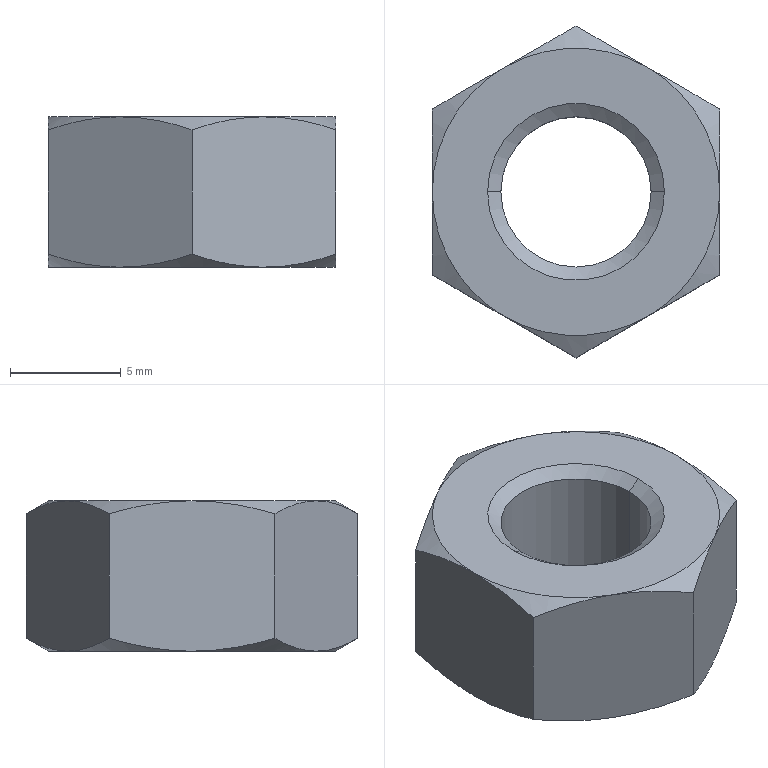Part | STEP file | Produce dryer cooling section-hex nut style 1_am_B18.2.4.1M - Hex nut, Style 1, M8 x 1.25 | 1 solid | 28 faces | box 13 x 15.011 x 6.8 mm | volume 737.453 mm3 | cone 16 | plane 8 | cylinder 4 | commonest cylinder face diameters 6.8 x2 8 x2
STEP:
#1=CARTESIAN_POINT('',(-4.,0.,-6.8));
#2=VERTEX_POINT('',#1);
#3=CARTESIAN_POINT('',(4.,0.,-6.8));
#4=VERTEX_POINT('',#3);
#5=CARTESIAN_POINT('',(0.,0.,-6.8));
#6=DIRECTION('',(0.,0.,1.));
#7=DIRECTION('',(-1.,0.,0.));
#8=AXIS2_PLACEMENT_3D('',#5,#6,#7);
#9=CIRCLE('',#8,4.);
#10=EDGE_CURVE('',#2,#4,#9,.T.);
#11=ORIENTED_EDGE('',*,*,#10,.F.);
#12=CARTESIAN_POINT('',(-4.,0.,-6.775));
#13=VERTEX_POINT('',#12);
#14=CARTESIAN_POINT('',(-4.,0.,-25.038));
#15=DIRECTION('',(0.,0.,1.));
#16=VECTOR('',#15,1000.);
#17=LINE('',#14,#16);
#18=EDGE_CURVE('',#2,#13,#17,.T.);
#19=ORIENTED_EDGE('',*,*,#18,.T.);
#20=CARTESIAN_POINT('',(4.,0.,-6.775));
#21=VERTEX_POINT('',#20);
#22=CARTESIAN_POINT('',(0.,0.,-6.775));
#23=DIRECTION('',(0.,0.,1.));
#24=DIRECTION('',(1.,0.,0.));
#25=AXIS2_PLACEMENT_3D('',#22,#23,#24);
#26=CIRCLE('',#25,4.);
#27=EDGE_CURVE('',#13,#21,#26,.T.);
#28=ORIENTED_EDGE('',*,*,#27,.T.);
#29=CARTESIAN_POINT('',(4.,0.,-25.038));
#30=DIRECTION('',(0.,0.,1.));
#31=VECTOR('',#30,1000.);
#32=LINE('',#29,#31);
#33=EDGE_CURVE('',#4,#21,#32,.T.);
#34=ORIENTED_EDGE('',*,*,#33,.F.);
#35=EDGE_LOOP('',(#11,#19,#28,#34));
#36=FACE_OUTER_BOUND('',#35,.T.);
#37=CARTESIAN_POINT('',(0.,0.,-25.038));
#38=DIRECTION('',(0.,0.,1.));
#39=DIRECTION('',(1.,0.,0.));
#40=AXIS2_PLACEMENT_3D('',#37,#38,#39);
#41=CYLINDRICAL_SURFACE('',#40,4.);
#42=ADVANCED_FACE('',(#36),#41,.F.);
#43=CARTESIAN_POINT('',(-3.4,0.,-6.354));
#44=VERTEX_POINT('',#43);
#45=CARTESIAN_POINT('',(3.4,0.,-6.354));
#46=VERTEX_POINT('',#45);
#47=CARTESIAN_POINT('',(0.,0.,-6.354));
#48=DIRECTION('',(0.,0.,1.));
#49=DIRECTION('',(-1.,0.,0.));
#50=AXIS2_PLACEMENT_3D('',#47,#48,#49);
#51=CIRCLE('',#50,3.4);
#52=EDGE_CURVE('',#44,#46,#51,.T.);
#53=ORIENTED_EDGE('',*,*,#52,.T.);
#54=CARTESIAN_POINT('',(4.,0.,-6.775));
#55=DIRECTION('',(0.8192,0.,-0.5736));
#56=VECTOR('',#55,1000.);
#57=LINE('',#54,#56);
#58=EDGE_CURVE('',#46,#21,#57,.T.);
#59=ORIENTED_EDGE('',*,*,#58,.T.);
#60=ORIENTED_EDGE('',*,*,#27,.F.);
#61=CARTESIAN_POINT('',(-4.,0.,-6.775));
#62=DIRECTION('',(-0.8192,0.,-0.5736));
#63=VECTOR('',#62,1000.);
#64=LINE('',#61,#63);
#65=EDGE_CURVE('',#44,#13,#64,.T.);
#66=ORIENTED_EDGE('',*,*,#65,.F.);
#67=EDGE_LOOP('',(#53,#59,#60,#66));
#68=FACE_OUTER_BOUND('',#67,.T.);
#69=CARTESIAN_POINT('',(0.,0.,-6.775));
#70=DIRECTION('',(0.,0.,-1.));
#71=DIRECTION('',(-1.,0.,0.));
#72=AXIS2_PLACEMENT_3D('',#69,#70,#71);
#73=CONICAL_SURFACE('',#72,4.,0.9599);
#74=ADVANCED_FACE('',(#68),#73,.F.);
#75=CARTESIAN_POINT('',(3.4,0.,-0.4201));
#76=VERTEX_POINT('',#75);
#77=CARTESIAN_POINT('',(-3.4,0.,-0.4201));
#78=VERTEX_POINT('',#77);
#79=CARTESIAN_POINT('',(0.,0.,-0.4201));
#80=DIRECTION('',(0.,0.,-1.));
#81=DIRECTION('',(1.,0.,0.));
#82=AXIS2_PLACEMENT_3D('',#79,#80,#81);
#83=CIRCLE('',#82,3.4);
#84=EDGE_CURVE('',#76,#78,#83,.T.);
#85=ORIENTED_EDGE('',*,*,#84,.T.);
#86=CARTESIAN_POINT('',(-4.,0.,0.));
#87=VERTEX_POINT('',#86);
#88=CARTESIAN_POINT('',(-3.34,0.,-0.4621));
#89=DIRECTION('',(-0.8192,0.,0.5736));
#90=VECTOR('',#89,1000.);
#91=LINE('',#88,#90);
#92=EDGE_CURVE('',#78,#87,#91,.T.);
#93=ORIENTED_EDGE('',*,*,#92,.T.);
#94=CARTESIAN_POINT('',(4.,0.,0.));
#95=VERTEX_POINT('',#94);
#96=CARTESIAN_POINT('',(0.,0.,0.));
#97=DIRECTION('',(0.,0.,1.));
#98=DIRECTION('',(1.,0.,0.));
#99=AXIS2_PLACEMENT_3D('',#96,#97,#98);
#100=CIRCLE('',#99,4.);
#101=EDGE_CURVE('',#87,#95,#100,.T.);
#102=ORIENTED_EDGE('',*,*,#101,.T.);
#103=CARTESIAN_POINT('',(3.34,0.,-0.4621));
#104=DIRECTION('',(0.8192,0.,0.5736));
#105=VECTOR('',#104,1000.);
#106=LINE('',#103,#105);
#107=EDGE_CURVE('',#76,#95,#106,.T.);
#108=ORIENTED_EDGE('',*,*,#107,.F.);
#109=EDGE_LOOP('',(#85,#93,#102,#108));
#110=FACE_OUTER_BOUND('',#109,.T.);
#111=CARTESIAN_POINT('',(0.,0.,-0.4621));
#112=DIRECTION('',(0.,0.,1.));
#113=DIRECTION('',(1.,0.,0.));
#114=AXIS2_PLACEMENT_3D('',#111,#112,#113);
#115=CONICAL_SURFACE('',#114,3.34,0.9599);
#116=ADVANCED_FACE('',(#110),#115,.F.);
#117=ORIENTED_EDGE('',*,*,#52,.F.);
#118=CARTESIAN_POINT('',(-3.4,0.,-6.8));
#119=DIRECTION('',(0.,0.,1.));
#120=VECTOR('',#119,1000.);
#121=LINE('',#118,#120);
#122=EDGE_CURVE('',#44,#78,#121,.T.);
#123=ORIENTED_EDGE('',*,*,#122,.T.);
#124=ORIENTED_EDGE('',*,*,#84,.F.);
#125=CARTESIAN_POINT('',(3.4,0.,-6.8));
#126=DIRECTION('',(0.,0.,1.));
#127=VECTOR('',#126,1000.);
#128=LINE('',#125,#127);
#129=EDGE_CURVE('',#46,#76,#128,.T.);
#130=ORIENTED_EDGE('',*,*,#129,.F.);
#131=EDGE_LOOP('',(#117,#123,#124,#130));
#132=FACE_OUTER_BOUND('',#131,.T.);
#133=CARTESIAN_POINT('',(0.,0.,-6.8));
#134=DIRECTION('',(0.,0.,1.));
#135=DIRECTION('',(1.,0.,0.));
#136=AXIS2_PLACEMENT_3D('',#133,#134,#135);
#137=CYLINDRICAL_SURFACE('',#136,3.4);
#138=ADVANCED_FACE('',(#132),#137,.F.);
#139=ORIENTED_EDGE('',*,*,#122,.F.);
#140=CARTESIAN_POINT('',(0.,0.,-6.354));
#141=DIRECTION('',(0.,0.,1.));
#142=DIRECTION('',(-1.,0.,0.));
#143=AXIS2_PLACEMENT_3D('',#140,#141,#142);
#144=CIRCLE('',#143,3.4);
#145=EDGE_CURVE('',#46,#44,#144,.T.);
#146=ORIENTED_EDGE('',*,*,#145,.F.);
#147=ORIENTED_EDGE('',*,*,#129,.T.);
#148=CARTESIAN_POINT('',(0.,0.,-0.4201));
#149=DIRECTION('',(0.,0.,-1.));
#150=DIRECTION('',(1.,0.,0.));
#151=AXIS2_PLACEMENT_3D('',#148,#149,#150);
#152=CIRCLE('',#151,3.4);
#153=EDGE_CURVE('',#78,#76,#152,.T.);
#154=ORIENTED_EDGE('',*,*,#153,.F.);
#155=EDGE_LOOP('',(#139,#146,#147,#154));
#156=FACE_OUTER_BOUND('',#155,.T.);
#157=CARTESIAN_POINT('',(0.,0.,-6.8));
#158=DIRECTION('',(0.,0.,1.));
#159=DIRECTION('',(1.,0.,0.));
#160=AXIS2_PLACEMENT_3D('',#157,#158,#159);
#161=CYLINDRICAL_SURFACE('',#160,3.4);
#162=ADVANCED_FACE('',(#156),#161,.F.);
#163=CARTESIAN_POINT('',(-6.5,3.753,-6.219));
#164=VERTEX_POINT('',#163);
#165=CARTESIAN_POINT('',(-6.5,3.753,-0.5806));
#166=VERTEX_POINT('',#165);
#167=CARTESIAN_POINT('',(-6.5,3.753,-6.8));
#168=DIRECTION('',(0.,0.,1.));
#169=VECTOR('',#168,1000.);
#170=LINE('',#167,#169);
#171=EDGE_CURVE('',#164,#166,#170,.T.);
#172=ORIENTED_EDGE('',*,*,#171,.T.);
#173=CARTESIAN_POINT('',(-3.25,5.629,0.));
#174=VERTEX_POINT('',#173);
#175=CARTESIAN_POINT('',(-6.5,3.753,-0.5806));
#176=CARTESIAN_POINT('',(-5.968,4.06,-0.4033));
#177=CARTESIAN_POINT('',(-5.433,4.369,-0.2573));
#178=CARTESIAN_POINT('',(-4.351,4.994,-0.05533));
#179=CARTESIAN_POINT('',(-3.804,5.309,0.));
#180=CARTESIAN_POINT('',(-3.25,5.629,0.));
#181=B_SPLINE_CURVE_WITH_KNOTS('',3,(#175,#176,#177,#178,#179,#180),.UNSPECIFIED.,.F.,.F.,(4,2,4),(0.000000238,0.001899,0.003797),.UNSPECIFIED.);
#182=EDGE_CURVE('',#166,#174,#181,.T.);
#183=ORIENTED_EDGE('',*,*,#182,.T.);
#184=CARTESIAN_POINT('',(0.,7.506,-0.5806));
#185=VERTEX_POINT('',#184);
#186=CARTESIAN_POINT('',(-3.25,5.629,0.));
#187=CARTESIAN_POINT('',(-2.974,5.788,0.));
#188=CARTESIAN_POINT('',(-2.697,5.948,-0.01372));
#189=CARTESIAN_POINT('',(-2.149,6.265,-0.06683));
#190=CARTESIAN_POINT('',(-1.877,6.422,-0.1062));
#191=CARTESIAN_POINT('',(-1.065,6.891,-0.2578));
#192=CARTESIAN_POINT('',(-0.5303,7.199,-0.4038));
#193=CARTESIAN_POINT('',(0.,7.506,-0.5806));
#194=B_SPLINE_CURVE_WITH_KNOTS('',3,(#186,#187,#188,#189,#190,#191,#192,#193),.UNSPECIFIED.,.F.,.F.,(4,2,2,4),(0.003797,0.004743,0.005689,0.00758),.UNSPECIFIED.);
#195=EDGE_CURVE('',#174,#185,#194,.T.);
#196=ORIENTED_EDGE('',*,*,#195,.T.);
#197=CARTESIAN_POINT('',(0.,7.506,-6.219));
#198=VERTEX_POINT('',#197);
#199=CARTESIAN_POINT('',(0.,7.506,-6.8));
#200=DIRECTION('',(0.,0.,1.));
#201=VECTOR('',#200,1000.);
#202=LINE('',#199,#201);
#203=EDGE_CURVE('',#198,#185,#202,.T.);
#204=ORIENTED_EDGE('',*,*,#203,.F.);
#205=CARTESIAN_POINT('',(-3.25,5.629,-6.8));
#206=VERTEX_POINT('',#205);
#207=CARTESIAN_POINT('',(-3.25,5.629,-6.8));
#208=CARTESIAN_POINT('',(-2.974,5.788,-6.8));
#209=CARTESIAN_POINT('',(-2.697,5.948,-6.786));
#210=CARTESIAN_POINT('',(-2.149,6.265,-6.733));
#211=CARTESIAN_POINT('',(-1.877,6.422,-6.694));
#212=CARTESIAN_POINT('',(-1.065,6.891,-6.542));
#213=CARTESIAN_POINT('',(-0.5303,7.199,-6.396));
#214=CARTESIAN_POINT('',(0.,7.506,-6.219));
#215=B_SPLINE_CURVE_WITH_KNOTS('',3,(#207,#208,#209,#210,#211,#212,#213,#214),.UNSPECIFIED.,.F.,.F.,(4,2,2,4),(0.003797,0.004743,0.005689,0.00758),.UNSPECIFIED.);
#216=EDGE_CURVE('',#206,#198,#215,.T.);
#217=ORIENTED_EDGE('',*,*,#216,.F.);
#218=CARTESIAN_POINT('',(-6.5,3.753,-6.219));
#219=CARTESIAN_POINT('',(-5.968,4.06,-6.397));
#220=CARTESIAN_POINT('',(-5.433,4.369,-6.543));
#221=CARTESIAN_POINT('',(-4.351,4.994,-6.745));
#222=CARTESIAN_POINT('',(-3.804,5.309,-6.8));
#223=CARTESIAN_POINT('',(-3.25,5.629,-6.8));
#224=B_SPLINE_CURVE_WITH_KNOTS('',3,(#218,#219,#220,#221,#222,#223),.UNSPECIFIED.,.F.,.F.,(4,2,4),(0.000000238,0.001899,0.003797),.UNSPECIFIED.);
#225=EDGE_CURVE('',#164,#206,#224,.T.);
#226=ORIENTED_EDGE('',*,*,#225,.F.);
#227=EDGE_LOOP('',(#172,#183,#196,#204,#217,#226));
#228=FACE_OUTER_BOUND('',#227,.T.);
#229=CARTESIAN_POINT('',(0.,7.506,-6.8));
#230=DIRECTION('',(-0.5,0.866,0.));
#231=DIRECTION('',(-0.866,-0.5,0.));
#232=AXIS2_PLACEMENT_3D('',#229,#230,#231);
#233=PLANE('',#232);
#234=ADVANCED_FACE('',(#228),#233,.T.);
#235=ORIENTED_EDGE('',*,*,#203,.T.);
#236=CARTESIAN_POINT('',(3.25,5.629,0.));
#237=VERTEX_POINT('',#236);
#238=CARTESIAN_POINT('',(0.,7.506,-0.5806));
#239=CARTESIAN_POINT('',(0.5317,7.199,-0.4033));
#240=CARTESIAN_POINT('',(1.067,6.889,-0.2573));
#241=CARTESIAN_POINT('',(2.149,6.265,-0.05533));
#242=CARTESIAN_POINT('',(2.696,5.949,0.));
#243=CARTESIAN_POINT('',(3.25,5.629,0.));
#244=B_SPLINE_CURVE_WITH_KNOTS('',3,(#238,#239,#240,#241,#242,#243),.UNSPECIFIED.,.F.,.F.,(4,2,4),(0.000000238,0.001899,0.003797),.UNSPECIFIED.);
#245=EDGE_CURVE('',#185,#237,#244,.T.);
#246=ORIENTED_EDGE('',*,*,#245,.T.);
#247=CARTESIAN_POINT('',(6.5,3.753,-0.5806));
#248=VERTEX_POINT('',#247);
#249=CARTESIAN_POINT('',(3.25,5.629,0.));
#250=CARTESIAN_POINT('',(3.526,5.47,0.));
#251=CARTESIAN_POINT('',(3.803,5.31,-0.01372));
#252=CARTESIAN_POINT('',(4.351,4.994,-0.06683));
#253=CARTESIAN_POINT('',(4.623,4.836,-0.1062));
#254=CARTESIAN_POINT('',(5.435,4.368,-0.2578));
#255=CARTESIAN_POINT('',(5.97,4.059,-0.4038));
#256=CARTESIAN_POINT('',(6.5,3.753,-0.5806));
#257=B_SPLINE_CURVE_WITH_KNOTS('',3,(#249,#250,#251,#252,#253,#254,#255,#256),.UNSPECIFIED.,.F.,.F.,(4,2,2,4),(0.003797,0.004743,0.005689,0.00758),.UNSPECIFIED.);
#258=EDGE_CURVE('',#237,#248,#257,.T.);
#259=ORIENTED_EDGE('',*,*,#258,.T.);
#260=CARTESIAN_POINT('',(6.5,3.753,-6.219));
#261=VERTEX_POINT('',#260);
#262=CARTESIAN_POINT('',(6.5,3.753,-6.8));
#263=DIRECTION('',(0.,0.,1.));
#264=VECTOR('',#263,1000.);
#265=LINE('',#262,#264);
#266=EDGE_CURVE('',#261,#248,#265,.T.);
#267=ORIENTED_EDGE('',*,*,#266,.F.);
#268=CARTESIAN_POINT('',(3.25,5.629,-6.8));
#269=VERTEX_POINT('',#268);
#270=CARTESIAN_POINT('',(3.25,5.629,-6.8));
#271=CARTESIAN_POINT('',(3.526,5.47,-6.8));
#272=CARTESIAN_POINT('',(3.803,5.31,-6.786));
#273=CARTESIAN_POINT('',(4.351,4.994,-6.733));
#274=CARTESIAN_POINT('',(4.623,4.836,-6.694));
#275=CARTESIAN_POINT('',(5.435,4.368,-6.542));
#276=CARTESIAN_POINT('',(5.97,4.059,-6.396));
#277=CARTESIAN_POINT('',(6.5,3.753,-6.219));
#278=B_SPLINE_CURVE_WITH_KNOTS('',3,(#270,#271,#272,#273,#274,#275,#276,#277),.UNSPECIFIED.,.F.,.F.,(4,2,2,4),(0.003797,0.004743,0.005689,0.00758),.UNSPECIFIED.);
#279=EDGE_CURVE('',#269,#261,#278,.T.);
#280=ORIENTED_EDGE('',*,*,#279,.F.);
#281=CARTESIAN_POINT('',(0.,7.506,-6.219));
#282=CARTESIAN_POINT('',(0.5317,7.199,-6.397));
#283=CARTESIAN_POINT('',(1.067,6.889,-6.543));
#284=CARTESIAN_POINT('',(2.149,6.265,-6.745));
#285=CARTESIAN_POINT('',(2.696,5.949,-6.8));
#286=CARTESIAN_POINT('',(3.25,5.629,-6.8));
#287=B_SPLINE_CURVE_WITH_KNOTS('',3,(#281,#282,#283,#284,#285,#286),.UNSPECIFIED.,.F.,.F.,(4,2,4),(0.000000238,0.001899,0.003797),.UNSPECIFIED.);
#288=EDGE_CURVE('',#198,#269,#287,.T.);
#289=ORIENTED_EDGE('',*,*,#288,.F.);
#290=EDGE_LOOP('',(#235,#246,#259,#267,#280,#289));
#291=FACE_OUTER_BOUND('',#290,.T.);
#292=CARTESIAN_POINT('',(6.5,3.753,-6.8));
#293=DIRECTION('',(0.5,0.866,0.));
#294=DIRECTION('',(-0.866,0.5,0.));
#295=AXIS2_PLACEMENT_3D('',#292,#293,#294);
#296=PLANE('',#295);
#297=ADVANCED_FACE('',(#291),#296,.T.);
#298=CARTESIAN_POINT('',(6.5,-3.753,-0.5806));
#299=VERTEX_POINT('',#298);
#300=CARTESIAN_POINT('',(6.5,0.,0.));
#301=VERTEX_POINT('',#300);
#302=CARTESIAN_POINT('',(6.5,-3.753,-0.5806));
#303=CARTESIAN_POINT('',(6.5,-3.142,-0.4044));
#304=CARTESIAN_POINT('',(6.5,-2.517,-0.2566));
#305=CARTESIAN_POINT('',(6.5,-1.264,-0.05451));
#306=CARTESIAN_POINT('',(6.5,-0.6342,0.));
#307=CARTESIAN_POINT('',(6.5,0.,0.));
#308=B_SPLINE_CURVE_WITH_KNOTS('',3,(#302,#303,#304,#305,#306,#307),.UNSPECIFIED.,.F.,.F.,(4,2,4),(0.006695,0.008594,0.01049),.UNSPECIFIED.);
#309=EDGE_CURVE('',#299,#301,#308,.T.);
#310=ORIENTED_EDGE('',*,*,#309,.F.);
#311=CARTESIAN_POINT('',(6.5,-3.753,-6.219));
#312=VERTEX_POINT('',#311);
#313=CARTESIAN_POINT('',(6.5,-3.753,-6.8));
#314=DIRECTION('',(0.,0.,1.));
#315=VECTOR('',#314,1000.);
#316=LINE('',#313,#315);
#317=EDGE_CURVE('',#312,#299,#316,.T.);
#318=ORIENTED_EDGE('',*,*,#317,.F.);
#319=CARTESIAN_POINT('',(6.5,0.,-6.8));
#320=VERTEX_POINT('',#319);
#321=CARTESIAN_POINT('',(6.5,-3.753,-6.219));
#322=CARTESIAN_POINT('',(6.5,-3.142,-6.396));
#323=CARTESIAN_POINT('',(6.5,-2.517,-6.543));
#324=CARTESIAN_POINT('',(6.5,-1.264,-6.745));
#325=CARTESIAN_POINT('',(6.5,-0.6342,-6.8));
#326=CARTESIAN_POINT('',(6.5,0.,-6.8));
#327=B_SPLINE_CURVE_WITH_KNOTS('',3,(#321,#322,#323,#324,#325,#326),.UNSPECIFIED.,.F.,.F.,(4,2,4),(0.006695,0.008594,0.01049),.UNSPECIFIED.);
#328=EDGE_CURVE('',#312,#320,#327,.T.);
#329=ORIENTED_EDGE('',*,*,#328,.T.);
#330=CARTESIAN_POINT('',(6.5,0.,-6.8));
#331=CARTESIAN_POINT('',(6.5,0.6345,-6.8));
#332=CARTESIAN_POINT('',(6.5,1.278,-6.744));
#333=CARTESIAN_POINT('',(6.5,2.531,-6.54));
#334=CARTESIAN_POINT('',(6.5,3.146,-6.395));
#335=CARTESIAN_POINT('',(6.5,3.753,-6.219));
#336=B_SPLINE_CURVE_WITH_KNOTS('',3,(#330,#331,#332,#333,#334,#335),.UNSPECIFIED.,.F.,.F.,(4,2,4),(0.01049,0.01239,0.01429),.UNSPECIFIED.);
#337=EDGE_CURVE('',#320,#261,#336,.T.);
#338=ORIENTED_EDGE('',*,*,#337,.T.);
#339=ORIENTED_EDGE('',*,*,#266,.T.);
#340=CARTESIAN_POINT('',(6.5,0.,0.));
#341=CARTESIAN_POINT('',(6.5,0.6345,0.));
#342=CARTESIAN_POINT('',(6.5,1.278,-0.05602));
#343=CARTESIAN_POINT('',(6.5,2.531,-0.2595));
#344=CARTESIAN_POINT('',(6.5,3.146,-0.4054));
#345=CARTESIAN_POINT('',(6.5,3.753,-0.5806));
#346=B_SPLINE_CURVE_WITH_KNOTS('',3,(#340,#341,#342,#343,#344,#345),.UNSPECIFIED.,.F.,.F.,(4,2,4),(0.01049,0.01239,0.01429),.UNSPECIFIED.);
#347=EDGE_CURVE('',#301,#248,#346,.T.);
#348=ORIENTED_EDGE('',*,*,#347,.F.);
#349=EDGE_LOOP('',(#310,#318,#329,#338,#339,#348));
#350=FACE_OUTER_BOUND('',#349,.T.);
#351=CARTESIAN_POINT('',(6.5,3.753,-6.8));
#352=DIRECTION('',(-1.,0.,0.));
#353=DIRECTION('',(0.,0.,1.));
#354=AXIS2_PLACEMENT_3D('',#351,#352,#353);
#355=PLANE('',#354);
#356=ADVANCED_FACE('',(#350),#355,.F.);
#357=ORIENTED_EDGE('',*,*,#317,.T.);
#358=CARTESIAN_POINT('',(3.25,-5.629,0.));
#359=VERTEX_POINT('',#358);
#360=CARTESIAN_POINT('',(6.5,-3.753,-0.5806));
#361=CARTESIAN_POINT('',(5.968,-4.06,-0.4033));
#362=CARTESIAN_POINT('',(5.433,-4.369,-0.2573));
#363=CARTESIAN_POINT('',(4.351,-4.994,-0.05533));
#364=CARTESIAN_POINT('',(3.804,-5.309,0.));
#365=CARTESIAN_POINT('',(3.25,-5.629,0.));
#366=B_SPLINE_CURVE_WITH_KNOTS('',3,(#360,#361,#362,#363,#364,#365),.UNSPECIFIED.,.F.,.F.,(4,2,4),(0.000000238,0.001899,0.003797),.UNSPECIFIED.);
#367=EDGE_CURVE('',#299,#359,#366,.T.);
#368=ORIENTED_EDGE('',*,*,#367,.T.);
#369=CARTESIAN_POINT('',(0.,-7.506,-0.5806));
#370=VERTEX_POINT('',#369);
#371=CARTESIAN_POINT('',(3.25,-5.629,0.));
#372=CARTESIAN_POINT('',(2.974,-5.788,0.));
#373=CARTESIAN_POINT('',(2.697,-5.948,-0.01372));
#374=CARTESIAN_POINT('',(2.149,-6.265,-0.06683));
#375=CARTESIAN_POINT('',(1.877,-6.422,-0.1062));
#376=CARTESIAN_POINT('',(1.065,-6.891,-0.2578));
#377=CARTESIAN_POINT('',(0.5303,-7.199,-0.4038));
#378=CARTESIAN_POINT('',(0.,-7.506,-0.5806));
#379=B_SPLINE_CURVE_WITH_KNOTS('',3,(#371,#372,#373,#374,#375,#376,#377,#378),.UNSPECIFIED.,.F.,.F.,(4,2,2,4),(0.003797,0.004743,0.005689,0.00758),.UNSPECIFIED.);
#380=EDGE_CURVE('',#359,#370,#379,.T.);
#381=ORIENTED_EDGE('',*,*,#380,.T.);
#382=CARTESIAN_POINT('',(0.,-7.506,-6.219));
#383=VERTEX_POINT('',#382);
#384=CARTESIAN_POINT('',(0.,-7.506,-6.8));
#385=DIRECTION('',(0.,0.,1.));
#386=VECTOR('',#385,1000.);
#387=LINE('',#384,#386);
#388=EDGE_CURVE('',#383,#370,#387,.T.);
#389=ORIENTED_EDGE('',*,*,#388,.F.);
#390=CARTESIAN_POINT('',(3.25,-5.629,-6.8));
#391=VERTEX_POINT('',#390);
#392=CARTESIAN_POINT('',(3.25,-5.629,-6.8));
#393=CARTESIAN_POINT('',(2.974,-5.788,-6.8));
#394=CARTESIAN_POINT('',(2.697,-5.948,-6.786));
#395=CARTESIAN_POINT('',(2.149,-6.265,-6.733));
#396=CARTESIAN_POINT('',(1.877,-6.422,-6.694));
#397=CARTESIAN_POINT('',(1.065,-6.891,-6.542));
#398=CARTESIAN_POINT('',(0.5303,-7.199,-6.396));
#399=CARTESIAN_POINT('',(0.,-7.506,-6.219));
#400=B_SPLINE_CURVE_WITH_KNOTS('',3,(#392,#393,#394,#395,#396,#397,#398,#399),.UNSPECIFIED.,.F.,.F.,(4,2,2,4),(0.003797,0.004743,0.005689,0.00758),.UNSPECIFIED.);
#401=EDGE_CURVE('',#391,#383,#400,.T.);
#402=ORIENTED_EDGE('',*,*,#401,.F.);
#403=CARTESIAN_POINT('',(6.5,-3.753,-6.219));
#404=CARTESIAN_POINT('',(5.968,-4.06,-6.397));
#405=CARTESIAN_POINT('',(5.433,-4.369,-6.543));
#406=CARTESIAN_POINT('',(4.351,-4.994,-6.745));
#407=CARTESIAN_POINT('',(3.804,-5.309,-6.8));
#408=CARTESIAN_POINT('',(3.25,-5.629,-6.8));
#409=B_SPLINE_CURVE_WITH_KNOTS('',3,(#403,#404,#405,#406,#407,#408),.UNSPECIFIED.,.F.,.F.,(4,2,4),(0.000000238,0.001899,0.003797),.UNSPECIFIED.);
#410=EDGE_CURVE('',#312,#391,#409,.T.);
#411=ORIENTED_EDGE('',*,*,#410,.F.);
#412=EDGE_LOOP('',(#357,#368,#381,#389,#402,#411));
#413=FACE_OUTER_BOUND('',#412,.T.);
#414=CARTESIAN_POINT('',(0.,-7.506,-6.8));
#415=DIRECTION('',(0.5,-0.866,0.));
#416=DIRECTION('',(0.866,0.5,0.));
#417=AXIS2_PLACEMENT_3D('',#414,#415,#416);
#418=PLANE('',#417);
#419=ADVANCED_FACE('',(#413),#418,.T.);
#420=ORIENTED_EDGE('',*,*,#388,.T.);
#421=CARTESIAN_POINT('',(-3.25,-5.629,0.));
#422=VERTEX_POINT('',#421);
#423=CARTESIAN_POINT('',(0.,-7.506,-0.5806));
#424=CARTESIAN_POINT('',(-0.5317,-7.199,-0.4033));
#425=CARTESIAN_POINT('',(-1.067,-6.889,-0.2573));
#426=CARTESIAN_POINT('',(-2.149,-6.265,-0.05533));
#427=CARTESIAN_POINT('',(-2.696,-5.949,0.));
#428=CARTESIAN_POINT('',(-3.25,-5.629,0.));
#429=B_SPLINE_CURVE_WITH_KNOTS('',3,(#423,#424,#425,#426,#427,#428),.UNSPECIFIED.,.F.,.F.,(4,2,4),(0.000000238,0.001899,0.003797),.UNSPECIFIED.);
#430=EDGE_CURVE('',#370,#422,#429,.T.);
#431=ORIENTED_EDGE('',*,*,#430,.T.);
#432=CARTESIAN_POINT('',(-6.5,-3.753,-0.5806));
#433=VERTEX_POINT('',#432);
#434=CARTESIAN_POINT('',(-3.25,-5.629,0.));
#435=CARTESIAN_POINT('',(-3.526,-5.47,0.));
#436=CARTESIAN_POINT('',(-3.803,-5.31,-0.01372));
#437=CARTESIAN_POINT('',(-4.351,-4.994,-0.06683));
#438=CARTESIAN_POINT('',(-4.623,-4.836,-0.1062));
#439=CARTESIAN_POINT('',(-5.435,-4.368,-0.2578));
#440=CARTESIAN_POINT('',(-5.97,-4.059,-0.4038));
#441=CARTESIAN_POINT('',(-6.5,-3.753,-0.5806));
#442=B_SPLINE_CURVE_WITH_KNOTS('',3,(#434,#435,#436,#437,#438,#439,#440,#441),.UNSPECIFIED.,.F.,.F.,(4,2,2,4),(0.003797,0.004743,0.005689,0.00758),.UNSPECIFIED.);
#443=EDGE_CURVE('',#422,#433,#442,.T.);
#444=ORIENTED_EDGE('',*,*,#443,.T.);
#445=CARTESIAN_POINT('',(-6.5,-3.753,-6.219));
#446=VERTEX_POINT('',#445);
#447=CARTESIAN_POINT('',(-6.5,-3.753,-6.8));
#448=DIRECTION('',(0.,0.,1.));
#449=VECTOR('',#448,1000.);
#450=LINE('',#447,#449);
#451=EDGE_CURVE('',#446,#433,#450,.T.);
#452=ORIENTED_EDGE('',*,*,#451,.F.);
#453=CARTESIAN_POINT('',(-3.25,-5.629,-6.8));
#454=VERTEX_POINT('',#453);
#455=CARTESIAN_POINT('',(-3.25,-5.629,-6.8));
#456=CARTESIAN_POINT('',(-3.526,-5.47,-6.8));
#457=CARTESIAN_POINT('',(-3.803,-5.31,-6.786));
#458=CARTESIAN_POINT('',(-4.351,-4.994,-6.733));
#459=CARTESIAN_POINT('',(-4.623,-4.836,-6.694));
#460=CARTESIAN_POINT('',(-5.435,-4.368,-6.542));
#461=CARTESIAN_POINT('',(-5.97,-4.059,-6.396));
#462=CARTESIAN_POINT('',(-6.5,-3.753,-6.219));
#463=B_SPLINE_CURVE_WITH_KNOTS('',3,(#455,#456,#457,#458,#459,#460,#461,#462),.UNSPECIFIED.,.F.,.F.,(4,2,2,4),(0.003797,0.004743,0.005689,0.00758),.UNSPECIFIED.);
#464=EDGE_CURVE('',#454,#446,#463,.T.);
#465=ORIENTED_EDGE('',*,*,#464,.F.);
#466=CARTESIAN_POINT('',(0.,-7.506,-6.219));
#467=CARTESIAN_POINT('',(-0.5317,-7.199,-6.397));
#468=CARTESIAN_POINT('',(-1.067,-6.889,-6.543));
#469=CARTESIAN_POINT('',(-2.149,-6.265,-6.745));
#470=CARTESIAN_POINT('',(-2.696,-5.949,-6.8));
#471=CARTESIAN_POINT('',(-3.25,-5.629,-6.8));
#472=B_SPLINE_CURVE_WITH_KNOTS('',3,(#466,#467,#468,#469,#470,#471),.UNSPECIFIED.,.F.,.F.,(4,2,4),(0.000000238,0.001899,0.003797),.UNSPECIFIED.);
#473=EDGE_CURVE('',#383,#454,#472,.T.);
#474=ORIENTED_EDGE('',*,*,#473,.F.);
#475=EDGE_LOOP('',(#420,#431,#444,#452,#465,#474));
#476=FACE_OUTER_BOUND('',#475,.T.);
#477=CARTESIAN_POINT('',(-6.5,-3.753,-6.8));
#478=DIRECTION('',(-0.5,-0.866,0.));
#479=DIRECTION('',(0.866,-0.5,0.));
#480=AXIS2_PLACEMENT_3D('',#477,#478,#479);
#481=PLANE('',#480);
#482=ADVANCED_FACE('',(#476),#481,.T.);
#483=ORIENTED_EDGE('',*,*,#451,.T.);
#484=CARTESIAN_POINT('',(-6.5,0.,0.));
#485=VERTEX_POINT('',#484);
#486=CARTESIAN_POINT('',(-6.5,-3.753,-0.5806));
#487=CARTESIAN_POINT('',(-6.5,-3.142,-0.4044));
#488=CARTESIAN_POINT('',(-6.5,-2.517,-0.2566));
#489=CARTESIAN_POINT('',(-6.5,-1.264,-0.05451));
#490=CARTESIAN_POINT('',(-6.5,-0.6342,0.));
#491=CARTESIAN_POINT('',(-6.5,0.,0.));
#492=B_SPLINE_CURVE_WITH_KNOTS('',3,(#486,#487,#488,#489,#490,#491),.UNSPECIFIED.,.F.,.F.,(4,2,4),(0.006695,0.008594,0.01049),.UNSPECIFIED.);
#493=EDGE_CURVE('',#433,#485,#492,.T.);
#494=ORIENTED_EDGE('',*,*,#493,.T.);
#495=CARTESIAN_POINT('',(-6.5,0.,0.));
#496=CARTESIAN_POINT('',(-6.5,0.6345,0.));
#497=CARTESIAN_POINT('',(-6.5,1.278,-0.05602));
#498=CARTESIAN_POINT('',(-6.5,2.531,-0.2595));
#499=CARTESIAN_POINT('',(-6.5,3.146,-0.4054));
#500=CARTESIAN_POINT('',(-6.5,3.753,-0.5806));
#501=B_SPLINE_CURVE_WITH_KNOTS('',3,(#495,#496,#497,#498,#499,#500),.UNSPECIFIED.,.F.,.F.,(4,2,4),(0.01049,0.01239,0.01429),.UNSPECIFIED.);
#502=EDGE_CURVE('',#485,#166,#501,.T.);
#503=ORIENTED_EDGE('',*,*,#502,.T.);
#504=ORIENTED_EDGE('',*,*,#171,.F.);
#505=CARTESIAN_POINT('',(-6.5,0.,-6.8));
#506=VERTEX_POINT('',#505);
#507=CARTESIAN_POINT('',(-6.5,0.,-6.8));
#508=CARTESIAN_POINT('',(-6.5,0.6345,-6.8));
#509=CARTESIAN_POINT('',(-6.5,1.278,-6.744));
#510=CARTESIAN_POINT('',(-6.5,2.531,-6.54));
#511=CARTESIAN_POINT('',(-6.5,3.146,-6.395));
#512=CARTESIAN_POINT('',(-6.5,3.753,-6.219));
#513=B_SPLINE_CURVE_WITH_KNOTS('',3,(#507,#508,#509,#510,#511,#512),.UNSPECIFIED.,.F.,.F.,(4,2,4),(0.01049,0.01239,0.01429),.UNSPECIFIED.);
#514=EDGE_CURVE('',#506,#164,#513,.T.);
#515=ORIENTED_EDGE('',*,*,#514,.F.);
#516=CARTESIAN_POINT('',(-6.5,-3.753,-6.219));
#517=CARTESIAN_POINT('',(-6.5,-3.142,-6.396));
#518=CARTESIAN_POINT('',(-6.5,-2.517,-6.543));
#519=CARTESIAN_POINT('',(-6.5,-1.264,-6.745));
#520=CARTESIAN_POINT('',(-6.5,-0.6342,-6.8));
#521=CARTESIAN_POINT('',(-6.5,0.,-6.8));
#522=B_SPLINE_CURVE_WITH_KNOTS('',3,(#516,#517,#518,#519,#520,#521),.UNSPECIFIED.,.F.,.F.,(4,2,4),(0.006695,0.008594,0.01049),.UNSPECIFIED.);
#523=EDGE_CURVE('',#446,#506,#522,.T.);
#524=ORIENTED_EDGE('',*,*,#523,.F.);
#525=EDGE_LOOP('',(#483,#494,#503,#504,#515,#524));
#526=FACE_OUTER_BOUND('',#525,.T.);
#527=CARTESIAN_POINT('',(-6.5,3.753,-6.8));
#528=DIRECTION('',(-1.,0.,0.));
#529=DIRECTION('',(0.,0.,1.));
#530=AXIS2_PLACEMENT_3D('',#527,#528,#529);
#531=PLANE('',#530);
#532=ADVANCED_FACE('',(#526),#531,.T.);
#533=CARTESIAN_POINT('',(0.,0.,0.));
#534=DIRECTION('',(0.,0.,1.));
#535=DIRECTION('',(1.,0.,0.));
#536=AXIS2_PLACEMENT_3D('',#533,#534,#535);
#537=CIRCLE('',#536,4.);
#538=EDGE_CURVE('',#95,#87,#537,.T.);
#539=ORIENTED_EDGE('',*,*,#538,.F.);
#540=ORIENTED_EDGE('',*,*,#101,.F.);
#541=EDGE_LOOP('',(#539,#540));
#542=FACE_BOUND('',#541,.T.);
#543=CARTESIAN_POINT('',(0.,0.,0.));
#544=DIRECTION('',(0.,0.,-1.));
#545=DIRECTION('',(-1.,0.,0.));
#546=AXIS2_PLACEMENT_3D('',#543,#544,#545);
#547=CIRCLE('',#546,6.5);
#548=EDGE_CURVE('',#485,#174,#547,.T.);
#549=ORIENTED_EDGE('',*,*,#548,.F.);
#550=CARTESIAN_POINT('',(0.,0.,0.));
#551=DIRECTION('',(0.,0.,-1.));
#552=DIRECTION('',(-1.,0.,0.));
#553=AXIS2_PLACEMENT_3D('',#550,#551,#552);
#554=CIRCLE('',#553,6.5);
#555=EDGE_CURVE('',#422,#485,#554,.T.);
#556=ORIENTED_EDGE('',*,*,#555,.F.);
#557=CARTESIAN_POINT('',(0.,0.,0.));
#558=DIRECTION('',(0.,0.,-1.));
#559=DIRECTION('',(-1.,0.,0.));
#560=AXIS2_PLACEMENT_3D('',#557,#558,#559);
#561=CIRCLE('',#560,6.5);
#562=EDGE_CURVE('',#359,#422,#561,.T.);
#563=ORIENTED_EDGE('',*,*,#562,.F.);
#564=CARTESIAN_POINT('',(0.,0.,0.));
#565=DIRECTION('',(0.,0.,-1.));
#566=DIRECTION('',(-1.,0.,0.));
#567=AXIS2_PLACEMENT_3D('',#564,#565,#566);
#568=CIRCLE('',#567,6.5);
#569=EDGE_CURVE('',#301,#359,#568,.T.);
#570=ORIENTED_EDGE('',*,*,#569,.F.);
#571=CARTESIAN_POINT('',(0.,0.,0.));
#572=DIRECTION('',(0.,0.,1.));
#573=DIRECTION('',(1.,0.,0.));
#574=AXIS2_PLACEMENT_3D('',#571,#572,#573);
#575=CIRCLE('',#574,6.5);
#576=EDGE_CURVE('',#301,#237,#575,.T.);
#577=ORIENTED_EDGE('',*,*,#576,.T.);
#578=CARTESIAN_POINT('',(0.,0.,0.));
#579=DIRECTION('',(0.,0.,-1.));
#580=DIRECTION('',(-1.,0.,0.));
#581=AXIS2_PLACEMENT_3D('',#578,#579,#580);
#582=CIRCLE('',#581,6.5);
#583=EDGE_CURVE('',#174,#237,#582,.T.);
#584=ORIENTED_EDGE('',*,*,#583,.F.);
#585=EDGE_LOOP('',(#549,#556,#563,#570,#577,#584));
#586=FACE_OUTER_BOUND('',#585,.T.);
#587=CARTESIAN_POINT('',(0.,7.506,0.));
#588=DIRECTION('',(0.,0.,-1.));
#589=DIRECTION('',(-1.,0.,0.));
#590=AXIS2_PLACEMENT_3D('',#587,#588,#589);
#591=PLANE('',#590);
#592=ADVANCED_FACE('',(#542,#586),#591,.F.);
#593=CARTESIAN_POINT('',(0.,0.,-6.8));
#594=DIRECTION('',(0.,0.,1.));
#595=DIRECTION('',(-1.,0.,0.));
#596=AXIS2_PLACEMENT_3D('',#593,#594,#595);
#597=CIRCLE('',#596,4.);
#598=EDGE_CURVE('',#4,#2,#597,.T.);
#599=ORIENTED_EDGE('',*,*,#598,.T.);
#600=ORIENTED_EDGE('',*,*,#10,.T.);
#601=EDGE_LOOP('',(#599,#600));
#602=FACE_BOUND('',#601,.T.);
#603=CARTESIAN_POINT('',(0.,0.,-6.8));
#604=DIRECTION('',(0.,0.,1.));
#605=DIRECTION('',(-1.,0.,0.));
#606=AXIS2_PLACEMENT_3D('',#603,#604,#605);
#607=CIRCLE('',#606,6.5);
#608=EDGE_CURVE('',#506,#454,#607,.T.);
#609=ORIENTED_EDGE('',*,*,#608,.F.);
#610=CARTESIAN_POINT('',(0.,0.,-6.8));
#611=DIRECTION('',(0.,0.,1.));
#612=DIRECTION('',(-1.,0.,0.));
#613=AXIS2_PLACEMENT_3D('',#610,#611,#612);
#614=CIRCLE('',#613,6.5);
#615=EDGE_CURVE('',#206,#506,#614,.T.);
#616=ORIENTED_EDGE('',*,*,#615,.F.);
#617=CARTESIAN_POINT('',(0.,0.,-6.8));
#618=DIRECTION('',(0.,0.,1.));
#619=DIRECTION('',(-1.,0.,0.));
#620=AXIS2_PLACEMENT_3D('',#617,#618,#619);
#621=CIRCLE('',#620,6.5);
#622=EDGE_CURVE('',#269,#206,#621,.T.);
#623=ORIENTED_EDGE('',*,*,#622,.F.);
#624=CARTESIAN_POINT('',(0.,0.,-6.8));
#625=DIRECTION('',(0.,0.,1.));
#626=DIRECTION('',(1.,0.,0.));
#627=AXIS2_PLACEMENT_3D('',#624,#625,#626);
#628=CIRCLE('',#627,6.5);
#629=EDGE_CURVE('',#320,#269,#628,.T.);
#630=ORIENTED_EDGE('',*,*,#629,.F.);
#631=CARTESIAN_POINT('',(0.,0.,-6.8));
#632=DIRECTION('',(0.,0.,1.));
#633=DIRECTION('',(-1.,0.,0.));
#634=AXIS2_PLACEMENT_3D('',#631,#632,#633);
#635=CIRCLE('',#634,6.5);
#636=EDGE_CURVE('',#391,#320,#635,.T.);
#637=ORIENTED_EDGE('',*,*,#636,.F.);
#638=CARTESIAN_POINT('',(0.,0.,-6.8));
#639=DIRECTION('',(0.,0.,1.));
#640=DIRECTION('',(-1.,0.,0.));
#641=AXIS2_PLACEMENT_3D('',#638,#639,#640);
#642=CIRCLE('',#641,6.5);
#643=EDGE_CURVE('',#454,#391,#642,.T.);
#644=ORIENTED_EDGE('',*,*,#643,.F.);
#645=EDGE_LOOP('',(#609,#616,#623,#630,#637,#644));
#646=FACE_OUTER_BOUND('',#645,.T.);
#647=CARTESIAN_POINT('',(0.,7.506,-6.8));
#648=DIRECTION('',(0.,0.,-1.));
#649=DIRECTION('',(-1.,0.,0.));
#650=AXIS2_PLACEMENT_3D('',#647,#648,#649);
#651=PLANE('',#650);
#652=ADVANCED_FACE('',(#602,#646),#651,.T.);
#653=ORIENTED_EDGE('',*,*,#225,.T.);
#654=ORIENTED_EDGE('',*,*,#615,.T.);
#655=ORIENTED_EDGE('',*,*,#514,.T.);
#656=EDGE_LOOP('',(#653,#654,#655));
#657=FACE_OUTER_BOUND('',#656,.T.);
#658=CARTESIAN_POINT('',(0.,0.,-6.8));
#659=DIRECTION('',(0.,0.,1.));
#660=DIRECTION('',(1.,0.,0.));
#661=AXIS2_PLACEMENT_3D('',#658,#659,#660);
#662=CONICAL_SURFACE('',#661,6.5,1.047);
#663=ADVANCED_FACE('',(#657),#662,.T.);
#664=ORIENTED_EDGE('',*,*,#216,.T.);
#665=ORIENTED_EDGE('',*,*,#288,.T.);
#666=ORIENTED_EDGE('',*,*,#622,.T.);
#667=EDGE_LOOP('',(#664,#665,#666));
#668=FACE_OUTER_BOUND('',#667,.T.);
#669=CARTESIAN_POINT('',(0.,0.,-6.8));
#670=DIRECTION('',(0.,0.,1.));
#671=DIRECTION('',(1.,0.,0.));
#672=AXIS2_PLACEMENT_3D('',#669,#670,#671);
#673=CONICAL_SURFACE('',#672,6.5,1.047);
#674=ADVANCED_FACE('',(#668),#673,.T.);
#675=ORIENTED_EDGE('',*,*,#279,.T.);
#676=ORIENTED_EDGE('',*,*,#337,.F.);
#677=ORIENTED_EDGE('',*,*,#629,.T.);
#678=EDGE_LOOP('',(#675,#676,#677));
#679=FACE_OUTER_BOUND('',#678,.T.);
#680=CARTESIAN_POINT('',(0.,0.,-6.8));
#681=DIRECTION('',(0.,0.,1.));
#682=DIRECTION('',(1.,0.,0.));
#683=AXIS2_PLACEMENT_3D('',#680,#681,#682);
#684=CONICAL_SURFACE('',#683,6.5,1.047);
#685=ADVANCED_FACE('',(#679),#684,.T.);
#686=ORIENTED_EDGE('',*,*,#410,.T.);
#687=ORIENTED_EDGE('',*,*,#636,.T.);
#688=ORIENTED_EDGE('',*,*,#328,.F.);
#689=EDGE_LOOP('',(#686,#687,#688));
#690=FACE_OUTER_BOUND('',#689,.T.);
#691=CARTESIAN_POINT('',(0.,0.,-6.8));
#692=DIRECTION('',(0.,0.,1.));
#693=DIRECTION('',(1.,0.,0.));
#694=AXIS2_PLACEMENT_3D('',#691,#692,#693);
#695=CONICAL_SURFACE('',#694,6.5,1.047);
#696=ADVANCED_FACE('',(#690),#695,.T.);
#697=ORIENTED_EDGE('',*,*,#401,.T.);
#698=ORIENTED_EDGE('',*,*,#473,.T.);
#699=ORIENTED_EDGE('',*,*,#643,.T.);
#700=EDGE_LOOP('',(#697,#698,#699));
#701=FACE_OUTER_BOUND('',#700,.T.);
#702=CARTESIAN_POINT('',(0.,0.,-6.8));
#703=DIRECTION('',(0.,0.,1.));
#704=DIRECTION('',(1.,0.,0.));
#705=AXIS2_PLACEMENT_3D('',#702,#703,#704);
#706=CONICAL_SURFACE('',#705,6.5,1.047);
#707=ADVANCED_FACE('',(#701),#706,.T.);
#708=ORIENTED_EDGE('',*,*,#464,.T.);
#709=ORIENTED_EDGE('',*,*,#523,.T.);
#710=ORIENTED_EDGE('',*,*,#608,.T.);
#711=EDGE_LOOP('',(#708,#709,#710));
#712=FACE_OUTER_BOUND('',#711,.T.);
#713=CARTESIAN_POINT('',(0.,0.,-6.8));
#714=DIRECTION('',(0.,0.,1.));
#715=DIRECTION('',(1.,0.,0.));
#716=AXIS2_PLACEMENT_3D('',#713,#714,#715);
#717=CONICAL_SURFACE('',#716,6.5,1.047);
#718=ADVANCED_FACE('',(#712),#717,.T.);
#719=ORIENTED_EDGE('',*,*,#555,.T.);
#720=ORIENTED_EDGE('',*,*,#493,.F.);
#721=ORIENTED_EDGE('',*,*,#443,.F.);
#722=EDGE_LOOP('',(#719,#720,#721));
#723=FACE_OUTER_BOUND('',#722,.T.);
#724=CARTESIAN_POINT('',(0.,0.,0.));
#725=DIRECTION('',(0.,0.,-1.));
#726=DIRECTION('',(-1.,0.,0.));
#727=AXIS2_PLACEMENT_3D('',#724,#725,#726);
#728=CONICAL_SURFACE('',#727,6.5,1.047);
#729=ADVANCED_FACE('',(#723),#728,.T.);
#730=ORIENTED_EDGE('',*,*,#562,.T.);
#731=ORIENTED_EDGE('',*,*,#430,.F.);
#732=ORIENTED_EDGE('',*,*,#380,.F.);
#733=EDGE_LOOP('',(#730,#731,#732));
#734=FACE_OUTER_BOUND('',#733,.T.);
#735=CARTESIAN_POINT('',(0.,0.,0.));
#736=DIRECTION('',(0.,0.,-1.));
#737=DIRECTION('',(-1.,0.,0.));
#738=AXIS2_PLACEMENT_3D('',#735,#736,#737);
#739=CONICAL_SURFACE('',#738,6.5,1.047);
#740=ADVANCED_FACE('',(#734),#739,.T.);
#741=ORIENTED_EDGE('',*,*,#309,.T.);
#742=ORIENTED_EDGE('',*,*,#569,.T.);
#743=ORIENTED_EDGE('',*,*,#367,.F.);
#744=EDGE_LOOP('',(#741,#742,#743));
#745=FACE_OUTER_BOUND('',#744,.T.);
#746=CARTESIAN_POINT('',(0.,0.,0.));
#747=DIRECTION('',(0.,0.,-1.));
#748=DIRECTION('',(-1.,0.,0.));
#749=AXIS2_PLACEMENT_3D('',#746,#747,#748);
#750=CONICAL_SURFACE('',#749,6.5,1.047);
#751=ADVANCED_FACE('',(#745),#750,.T.);
#752=ORIENTED_EDGE('',*,*,#576,.F.);
#753=ORIENTED_EDGE('',*,*,#347,.T.);
#754=ORIENTED_EDGE('',*,*,#258,.F.);
#755=EDGE_LOOP('',(#752,#753,#754));
#756=FACE_OUTER_BOUND('',#755,.T.);
#757=CARTESIAN_POINT('',(0.,0.,0.));
#758=DIRECTION('',(0.,0.,-1.));
#759=DIRECTION('',(-1.,0.,0.));
#760=AXIS2_PLACEMENT_3D('',#757,#758,#759);
#761=CONICAL_SURFACE('',#760,6.5,1.047);
#762=ADVANCED_FACE('',(#756),#761,.T.);
#763=ORIENTED_EDGE('',*,*,#583,.T.);
#764=ORIENTED_EDGE('',*,*,#245,.F.);
#765=ORIENTED_EDGE('',*,*,#195,.F.);
#766=EDGE_LOOP('',(#763,#764,#765));
#767=FACE_OUTER_BOUND('',#766,.T.);
#768=CARTESIAN_POINT('',(0.,0.,0.));
#769=DIRECTION('',(0.,0.,-1.));
#770=DIRECTION('',(-1.,0.,0.));
#771=AXIS2_PLACEMENT_3D('',#768,#769,#770);
#772=CONICAL_SURFACE('',#771,6.5,1.047);
#773=ADVANCED_FACE('',(#767),#772,.T.);
#774=ORIENTED_EDGE('',*,*,#502,.F.);
#775=ORIENTED_EDGE('',*,*,#548,.T.);
#776=ORIENTED_EDGE('',*,*,#182,.F.);
#777=EDGE_LOOP('',(#774,#775,#776));
#778=FACE_OUTER_BOUND('',#777,.T.);
#779=CARTESIAN_POINT('',(0.,0.,0.));
#780=DIRECTION('',(0.,0.,-1.));
#781=DIRECTION('',(-1.,0.,0.));
#782=AXIS2_PLACEMENT_3D('',#779,#780,#781);
#783=CONICAL_SURFACE('',#782,6.5,1.047);
#784=ADVANCED_FACE('',(#778),#783,.T.);
#785=ORIENTED_EDGE('',*,*,#92,.F.);
#786=ORIENTED_EDGE('',*,*,#153,.T.);
#787=ORIENTED_EDGE('',*,*,#107,.T.);
#788=ORIENTED_EDGE('',*,*,#538,.T.);
#789=EDGE_LOOP('',(#785,#786,#787,#788));
#790=FACE_OUTER_BOUND('',#789,.T.);
#791=CARTESIAN_POINT('',(0.,0.,-0.4621));
#792=DIRECTION('',(0.,0.,1.));
#793=DIRECTION('',(1.,0.,0.));
#794=AXIS2_PLACEMENT_3D('',#791,#792,#793);
#795=CONICAL_SURFACE('',#794,3.34,0.9599);
#796=ADVANCED_FACE('',(#790),#795,.F.);
#797=ORIENTED_EDGE('',*,*,#58,.F.);
#798=ORIENTED_EDGE('',*,*,#145,.T.);
#799=ORIENTED_EDGE('',*,*,#65,.T.);
#800=CARTESIAN_POINT('',(0.,0.,-6.775));
#801=DIRECTION('',(0.,0.,1.));
#802=DIRECTION('',(1.,0.,0.));
#803=AXIS2_PLACEMENT_3D('',#800,#801,#802);
#804=CIRCLE('',#803,4.);
#805=EDGE_CURVE('',#21,#13,#804,.T.);
#806=ORIENTED_EDGE('',*,*,#805,.F.);
#807=EDGE_LOOP('',(#797,#798,#799,#806));
#808=FACE_OUTER_BOUND('',#807,.T.);
#809=CARTESIAN_POINT('',(0.,0.,-6.775));
#810=DIRECTION('',(0.,0.,-1.));
#811=DIRECTION('',(-1.,0.,0.));
#812=AXIS2_PLACEMENT_3D('',#809,#810,#811);
#813=CONICAL_SURFACE('',#812,4.,0.9599);
#814=ADVANCED_FACE('',(#808),#813,.F.);
#815=ORIENTED_EDGE('',*,*,#18,.F.);
#816=ORIENTED_EDGE('',*,*,#598,.F.);
#817=ORIENTED_EDGE('',*,*,#33,.T.);
#818=ORIENTED_EDGE('',*,*,#805,.T.);
#819=EDGE_LOOP('',(#815,#816,#817,#818));
#820=FACE_OUTER_BOUND('',#819,.T.);
#821=CARTESIAN_POINT('',(0.,0.,-25.038));
#822=DIRECTION('',(0.,0.,1.));
#823=DIRECTION('',(1.,0.,0.));
#824=AXIS2_PLACEMENT_3D('',#821,#822,#823);
#825=CYLINDRICAL_SURFACE('',#824,4.);
#826=ADVANCED_FACE('',(#820),#825,.F.);
#827=CLOSED_SHELL('',(#42,#74,#116,#138,#162,#234,#297,#356,#419,#482,#532,#592,#652,#663,#674,#685,#696,#707,#718,#729,#740,#751,#762,#773,#784,#796,#814,#826));
#828=MANIFOLD_SOLID_BREP('',#827);
#829=CARTESIAN_POINT('',(0.,0.,0.));
#830=DIRECTION('',(0.,0.,1.));
#831=DIRECTION('',(1.,0.,0.));
#832=AXIS2_PLACEMENT_3D('',#829,#830,#831);
#833=(LENGTH_UNIT()NAMED_UNIT(*)SI_UNIT(.MILLI.,.METRE.));
#834=UNCERTAINTY_MEASURE_WITH_UNIT(LENGTH_MEASURE(0.00001),#833,'','');
#835=(NAMED_UNIT(*)PLANE_ANGLE_UNIT()SI_UNIT($,.RADIAN.));
#836=(NAMED_UNIT(*)SI_UNIT($,.STERADIAN.)SOLID_ANGLE_UNIT());
#837=(GEOMETRIC_REPRESENTATION_CONTEXT(3)GLOBAL_UNCERTAINTY_ASSIGNED_CONTEXT((#834))GLOBAL_UNIT_ASSIGNED_CONTEXT((#833,#835,#836))REPRESENTATION_CONTEXT('',''));
#838=ADVANCED_BREP_SHAPE_REPRESENTATION('',(#828,#832),#837);